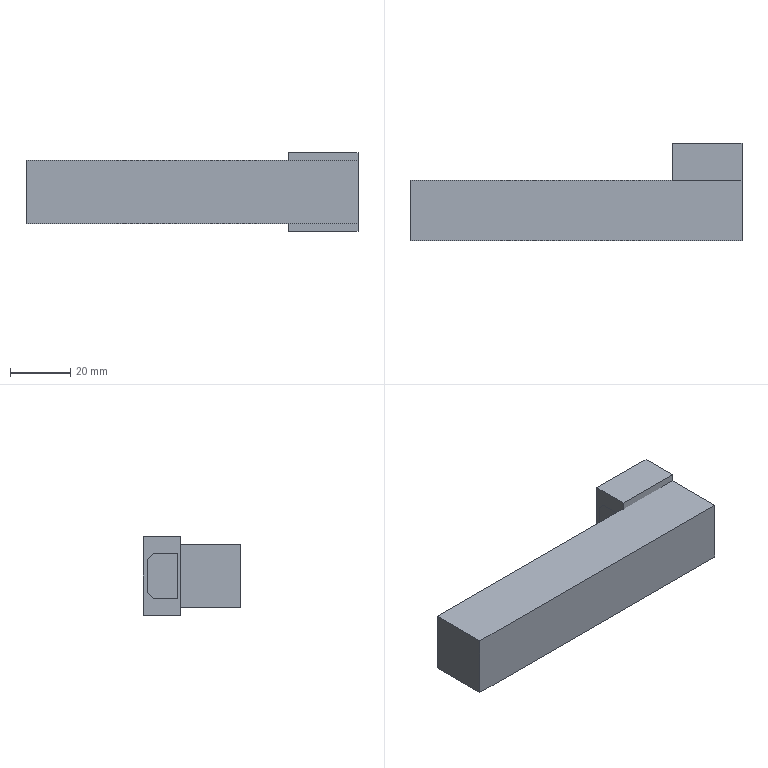NC program | NX | posted with a generic post | part box 110 x 32.2 x 26 mm
Lines 1 to 2298 of 5595, first 1795 of 2282 lines:
N10 G17 G21 G94 G90
(PLANAR_MILL , TOOL : D16C)
N12 T01 M6
N14 G54
N16 G17 G0 G90 X-64.06 Y0.06 S2300 M3
N18 G43 Z20. H1
N20 Z3.
N22 G94 G1 Z0. F800.
N24 X-48.06
N26 X50.
N28 X66.
N30 Z3.
N32 G0 Z20.
(ADAPTIVE_MILLING , TOOL : D16C)
N34 X-47.639 Y-25.487 S3500
N36 Z-9.3
N38 G1 X-47.612 Y-25.339 Z-10.237 F1500.
N40 X-47.586 Y-25.191 Z-10.608
N42 X-47.559 Y-25.044 Z-10.88
N44 X-47.533 Y-24.896 Z-11.1
N46 X-47.506 Y-24.748 Z-11.284
N48 X-47.48 Y-24.601 Z-11.442
N50 X-47.453 Y-24.453 Z-11.58
N52 X-47.427 Y-24.306 Z-11.7
N54 X-47.4 Y-24.158 Z-11.805
N56 X-47.374 Y-24.01 Z-11.898
N58 X-47.348 Y-23.863 Z-11.979
N60 X-47.321 Y-23.715 Z-12.05
N62 X-47.295 Y-23.567 Z-12.11
N64 X-47.268 Y-23.42 Z-12.162
N66 X-47.242 Y-23.272 Z-12.205
N68 X-47.215 Y-23.124 Z-12.239
N70 X-47.189 Y-22.977 Z-12.266
N72 X-47.162 Y-22.829 Z-12.285
N74 X-47.136 Y-22.681 Z-12.296
N76 X-47.109 Y-22.534 Z-12.3
N78 X-46.726 Y-20.396
N80 G3 X-48.19 Y-18.5 R1.616
N82 X-52.507 Y-18.235 R31.569
N84 G2 X-59.562 Y-14.889 R8.829
N86 X-62.127 Y-9.164 R12.797
N88 X-62.649 Y-3.232 R34.866
N90 X-62.685 Y8.843 R655.168
N92 X-59.143 Y15.242 R8.906
N94 X-53.354 Y17.682 R13.135
N96 X-47.117 Y18.161 R39.093
N98 X-37.067 Y18.2 R709.403
N100 G1 X52.988 Y18.199
N102 G2 X59.48 Y14.958 R8.794
N104 X62.125 Y9.144 R12.723
N106 X62.646 Y3.325 R34.318
N108 X62.685 Y-8.824 R620.01
N110 X59.165 Y-15.219 R8.912
N112 X53.418 Y-17.669 R13.064
N114 X47.519 Y-18.153 R36.787
N116 X37.019 Y-18.2 R709.315
N118 G1 X-45.793 Y-18.198
N120 G2 X-51.751 Y-17.939 R361.241
N122 X-59.844 Y-12.708 R10.728
N124 X-61.93 Y-6.607 R16.222
N126 X-62.365 Y0.274 R52.
N128 X-62.375 Y6.948 R189.513
N130 X-57.397 Y15.19 R10.59
N132 X-51.118 Y17.421 R15.907
N134 X-44.312 Y17.862 R50.704
N136 X-34.038 Y17.899 R728.543
N138 G1 X50.764
N140 G2 X59.63 Y12.987 R10.568
N142 X61.889 Y6.819 R15.681
N144 X62.357 Y0.203 R47.136
N146 X62.368 Y-7.033 R152.163
N148 X57.353 Y-15.217 R10.608
N150 X51.243 Y-17.401 R15.846
N152 X44.327 Y-17.862 R49.567
N154 X34.802 Y-17.899 R695.67
N156 G1 X-44.363 Y-17.897
N158 G2 X-50.474 Y-17.659 R87.545
N160 X-59.671 Y-11.376 R11.886
N162 X-61.657 Y-4.886 R18.515
N164 X-62.073 Y2.861 R65.244
N166 X-61.929 Y6.64 R22.837
N168 X-55.949 Y15.085 R11.728
N170 X-49.444 Y17.14 R18.144
N172 X-42.111 Y17.564 R60.452
N174 G1 X-31.761 Y17.599
N176 X48.813
N178 G2 X56.36 Y15.207 R11.928
N180 X60.794 Y8.696 R13.349
N182 X61.906 Y2.283 R25.894
N184 X62.05 Y-5.513 R87.082
N186 X56.042 Y-15.03 R11.703
N188 X49.505 Y-17.131 R17.992
N190 X42.06 Y-17.565 R60.128
N192 G1 X31.785 Y-17.599
N194 X-44.515 Y-17.588
N196 G2 X-49.457 Y-17.36 R55.401
N198 X-59.419 Y-10.311 R12.761
N200 X-61.353 Y-3.606 R20.225
N202 X-61.706 Y4.366 R51.532
N204 X-55.08 Y14.719 R12.499
N206 X-48.31 Y16.814 R19.379
N208 X-40.94 Y17.256 R62.006
N210 X-29.84 Y17.298 R749.749
N212 G1 X47.387 Y17.297
N214 G2 X53.58 Y16.029 R14.025
N216 X59.745 Y9.539 R13.034
N218 X61.431 Y2.877 R21.689
N220 X61.701 Y-4.424 R50.131
N222 X54.99 Y-14.767 R12.509
N224 X48.317 Y-16.812 R19.469
N226 X40.91 Y-17.256 R62.113
N228 X29.81 Y-17.298 R750.3
N230 G1 X-43.94 Y-17.299
N232 G2 X-48.686 Y-17.038 R42.716
N234 X-59.106 Y-9.454 R13.461
N236 X-61.044 Y-2.515 R21.574
N238 X-61.313 Y3.658 R33.117
N240 X-54.289 Y14.363 R13.08
N242 X-47.321 Y16.489 R20.415
N244 X-39.165 Y16.959 R67.725
N246 X-29.04 Y16.998 R721.188
N248 G1 X46.158 Y16.995
N250 G2 X51.97 Y16.024 R16.081
N252 X59.155 Y9.24 R13.423
N254 X61.051 Y2.363 R21.636
N256 X61.313 Y-3.623 R32.621
N258 X54.248 Y-14.384 R13.087
N260 X51.218 Y-15.664 R12.421
N262 X44.162 Y-16.796 R30.617
N264 X33.215 Y-16.995 R202.408
N266 G1 X28.115 Y-16.998
N268 X-43.948
N270 G2 X-49.108 Y-16.502 R26.27
N272 X-58.683 Y-8.888 R13.993
N274 X-60.688 Y-1.889 R22.084
N276 X-60.752 Y4.127 R20.912
N278 X-53.818 Y13.867 R13.457
N280 X-46.89 Y16.097 R20.532
N282 X-38.852 Y16.642 R61.265
N284 X-26.552 Y16.698 R765.35
N286 G1 X45.67 Y16.69
N288 G2 X52.27 Y15.251 R16.557
N290 G1 X52.52 Y15.191
N292 G2 X54.791 Y14.033 R9.495
N294 X57.268 Y11.365 R11.153
N296 X60.403 Y3.621 R19.669
N298 X60.886 Y-2.98 R25.727
N300 X57.099 Y-11.412 R13.467
N302 X54.022 Y-14.504 R7.94
N304 G1 X53.699 Y-14.702
N306 G2 X51.274 Y-15.49 R9.495
N308 X40.212 Y-16.618 R60.834
N310 X26.563 Y-16.698 R718.931
N312 G1 X-43.925
N314 G2 X-49.727 Y-15.818 R21.169
N316 X-58.348 Y-8.202 R14.524
N318 X-60.419 Y2.472 R21.678
N320 X-54.064 Y12.97 R13.725
N322 G1 X-52.849 Y14.034
N324 G2 X-50.577 Y15.191 R9.495
N326 X-48.103 Y15.65 R13.193
N328 X-37.295 Y16.35 R87.284
N330 X-25.146 Y16.397 R783.974
N332 G1 X44.995 Y16.396
N334 G2 X49.944 Y15.596 R22.073
N336 G1 X51.276 Y15.489
N338 X52.297 Y15.244
N340 G3 X53.497 Y15.43 R1.602
N342 G1 X54.112 Y15.801
N344 X56.844 Y17.447 Z-12.2
N346 G2 X57.413 Y17.739 R2.603 F15000.
N348 X59.229 Y17.101 R1.6
N350 G1 X62.55 Y12.119
N352 G2 X64.187 Y8.556 R12.517
N354 X65.082 Y4.692 R44.004
N356 G1 X65.33 Y3.355
N358 X65.564 Y2.016
N360 G2 X65.447 Y-5.571 R23.318
N362 X61.974 Y-13.417 R17.115
N364 G1 X57.488 Y-19.078
N366 G2 X54.972 Y-19.068 R1.6
N368 G1 X54.646 Y-18.649
N370 X52.686 Y-16.133 Z-12.3 F1500.
N372 G3 X51.274 Y-15.49 R1.603
N374 X45.161 Y-16.045 R728.767
N376 G2 X33.243 Y-16.386 R166.247
N378 G1 X25.293 Y-16.397
N380 X-43.919 Y-16.398
N382 G2 X-49.12 Y-15.508 R24.023
N384 X-50.58 Y-15.191 R10.043
N386 X-52.974 Y-13.946 R9.488
N388 X-55.554 Y-11.472 R18.869
N390 X-57.628 Y-8.549 R10.409
N392 X-59.955 Y1.385 R20.353
N394 X-57.372 Y8.945 R13.999
N396 X-56.593 Y10.291 R9.876
N398 G1 X-55.763 Y11.263
N400 X-53.986 Y13.04
N402 G3 X-54.851 Y15.749 R1.6
N404 X-55.855 Y15.599 Z-12.268 R1.733
N406 G1 X-57.859 Y14.797 Z-12.2
N408 X-60.326 Y13.81 F15000.
N410 G3 X-61.162 Y13.04 R1.603
N412 G1 X-61.98 Y11.408
N414 X-62.786 Y9.77
N416 G3 X-64.757 Y2.588 R23.064
N418 X-64.582 Y-2.243 R18.278
N420 G1 X-63.526 Y-8.432
N422 G3 X-62.902 Y-9.448 R1.602
N424 G1 X-60.84 Y-10.979
N426 X-58.912 Y-12.41 Z-12.275 F1500.
N428 G3 X-58.191 Y-12.708 Z-12.3 R1.615
N430 X-56.594 Y-10.289 R1.6
N432 G2 X-57.751 Y-8.017 R9.495
N434 X-59.297 Y-2.109 R31.269
N436 X-58.111 Y6.47 R15.528
N438 G1 X-58.059 Y6.689
N440 G3 X-59.751 Y8.499 R1.6
N442 X-60.887 Y7.911 Z-12.259 R1.617
N444 G1 X-62.067 Y6.456 Z-12.2
N446 X-63.918 Y4.174 F15000.
N448 G3 X-64.274 Y3.101 R1.603
N450 G1 X-63.966 Y-4.429
N452 G3 X-63.641 Y-5.332 R1.606
N454 G1 X-61.967 Y-7.535
N456 X-60.523 Y-9.427 Z-12.275 F1500.
N458 G3 X-59.87 Y-9.888 Z-12.3 R1.605
N460 X-57.751 Y-8.017 R1.6
N462 G2 X-58.869 Y-2.323 R50.127
N464 X-58.379 Y4.108 R17.226
N466 G3 X-58.15 Y5.501 R4.5
N468 G2 X-57.751 Y8.02 R9.498
N470 G1 X-57.334 Y9.024
N472 G3 X-59.89 Y10.82 R1.6
N474 G1 X-60.105 Y10.579 Z-12.29
N476 X-60.294 Y10.319 Z-12.28
N478 X-61.788 Y8.259 Z-12.2
N480 X-63.25 Y6.243 F15000.
N482 G3 X-63.549 Y5.436 R1.61
N484 G1 X-64.264 Y-3.186
N486 G3 X-63.892 Y-4.35 R1.602
N488 G1 X-62.082 Y-6.493
N490 X-61.446 Y-7.249 Z-12.231 F1500.
N492 X-60.803 Y-7.999 Z-12.262
N494 G3 X-59.73 Y-8.497 Z-12.3 R1.6
N496 X-58.05 Y-6.774 R1.6
N498 X-58.467 Y-2.9 R167.508
N500 G2 X-58.153 Y3.155 R23.608
N502 G1 X-58.15 Y5.199
N504 G3 X-59.745 Y6.799 R1.6
N506 X-60.973 Y6.231 Z-12.256 R1.612
N508 G1 X-62.129 Y4.861 Z-12.2
N510 X-63.987 Y2.659 F15000.
N512 G3 X-64.365 Y1.611 R1.603
N514 G1 X-64.323 Y-2.438
N516 G3 X-63.967 Y-3.428 R1.604
N518 G1 X-62.14 Y-5.686
N520 X-60.885 Y-7.227 Z-12.262 F1500.
N522 G3 X-59.833 Y-7.746 Z-12.3 R1.6
N524 X-58.109 Y-6.026 R1.6
N526 G2 X-58.172 Y-3.893 R34.44
N528 X-58.15 Y0.129 R34.348
N530 G1 Y3.241
N532 G3 X-59.75 Y4.841 R1.6
N534 X-60.975 Y4.271 Z-12.256 R1.612
N536 G1 X-62.129 Y2.897 Z-12.2
N538 X-63.99 Y0.683 F15000.
N540 G3 X-64.365 Y-0.347 R1.603
N542 G1 X-64.367 Y-0.847
N544 X-64.354 Y-1.347
N546 G3 X-63.99 Y-2.191 R1.607
N548 G1 X-62.148 Y-4.383
N550 X-61.533 Y-5.12 Z-12.23 F1500.
N552 X-60.908 Y-5.849 Z-12.26
N554 G3 X-59.779 Y-6.349 Z-12.3 R1.599
N556 X-58.15 Y-4.749 R1.6
N558 G1 Y5.501
N560 G2 X-57.751 Y8.02 R9.498
N562 X-56.593 Y10.291 R9.495
N564 G1 X-55.763 Y11.263
N566 X-53.822 Y13.203
N568 G2 X-51.759 Y14.702 R9.498
N570 X-49.334 Y15.49 R9.495
N572 X-46.196 Y15.655 R64.482
N574 X-31.016 Y16.089 R214.997
N576 G1 X-23.966 Y16.097
N578 X43.658 Y16.09
N580 G2 X48.257 Y15.59 R33.158
N582 G1 X50.001
N584 G3 X51.59 Y17.372 R1.6
N586 X50.933 Y18.49 Z-12.258 R1.617
N588 G1 X49.426 Y19.57 Z-12.2
N590 X47.811 Y20.728 F15000.
N592 G3 X46.861 Y21.028 R1.605
N594 G1 X-43.282 Y20.03
N596 X-43.489 Y20.012
N598 X-43.693 Y19.972
N600 X-45.099 Y19.58
N602 X-48.172 Y18.725 Z-12.3 F1500.
N604 G3 X-47.722 Y15.59 R1.6
N606 X-37.447 Y15.727 R305.695
N608 G2 X-22.972 Y15.797 R829.663
N610 G1 X44.428 Y15.796
N612 X46.077 Y15.59
N614 X48.289
N616 G3 X48.775 Y18.714 R1.6
N618 G1 X45.704 Y19.573 Z-12.2
N620 X44.922 Y19.794 F15000.
N622 X44.138 Y20.004
N624 X43.849 Y20.03
N626 X-39.232
N628 X-39.449 Y20.013
N630 X-39.662 Y19.971
N632 X-41.059 Y19.581
N634 X-44.131 Y18.723 Z-12.3 F1500.
N636 G3 X-43.672 Y15.59 R1.6
N638 G1 X50.001
N640 G2 X52.52 Y15.191 R9.498
N642 X54.791 Y14.033 R9.495
N644 X56.594 Y12.229 R9.495
N646 X58.612 Y8.215 R22.088
N648 X60.474 Y-1.783 R25.602
N650 X58.204 Y-9.005 R14.567
N652 G3 X57.8 Y-9.765 R4.628
N654 X58.945 Y-11.766 R1.6
N656 X60.275 Y-11.509 Z-12.256 R1.612
N658 G1 X61.724 Y-10.458 Z-12.2
N660 X64.153 Y-8.697 F15000.
N662 G3 X64.731 Y-7.908 R1.605
N664 G1 X65.118 Y-6.757
N666 X65.489 Y-5.6
N668 G3 X65.727 Y-2.15 R8.614
N670 G1 X64.194 Y9.282
N672 G3 X63.52 Y10.384 R1.602
N674 G1 X61.247 Y11.96
N676 X59.576 Y13.112 Z-12.264 F1500.
N678 G3 X58.463 Y13.327 Z-12.3 R1.6
N680 X57.262 Y11.139 R1.6
N682 G2 X58.592 Y7.424 R35.54
N684 X60.011 Y-0.144 R27.732
N686 X58.547 Y-7.21 R16.254
N688 G3 X58.067 Y-8.5 R6.221
N690 X59.065 Y-10.155 R1.6
N692 X60.42 Y-10.076 Z-12.256 R1.612
N694 G1 X61.992 Y-9.224 Z-12.2
N696 X64.161 Y-8.049 F15000.
N698 G3 X64.999 Y-6.642 R1.601
N700 G1 Y-1.24
N702 G3 X64.482 Y3.85 R25.383
N704 G1 X63.966 Y6.369
N706 G3 X63.696 Y6.984 R1.625
N708 G1 X61.994 Y9.342
N710 X60.554 Y11.331 Z-12.277 F1500.
N712 G3 X59.983 Y11.781 Z-12.3 R1.61
N714 X57.751 Y9.957 R1.6
N716 G2 X59.123 Y4.086 R181.863
N718 X58.537 Y-5.901 R18.835
N720 G3 X58.15 Y-7.362 R7.624
N722 G2 X57.751 Y-9.96 R9.467
N724 G1 X57.261 Y-11.141
N726 X57.046 Y-11.493
N728 G3 X59.742 Y-13.215 R1.6
N730 G1 X60.044 Y-12.76
N732 X61.811 Y-10.105 Z-12.2
N734 X63.213 Y-7.992 F15000.
N736 X63.774 Y-6.885
N738 X64.316 Y-5.769
N740 G3 X64.88 Y-2.352 R7.126
N742 G1 X64.264 Y5.126
N744 G3 X63.927 Y5.984 R1.607
N746 G1 X62.089 Y8.32
N748 X60.842 Y9.897 Z-12.263 F1500.
N750 G3 X59.822 Y10.429 Z-12.3 R1.6
N752 X58.05 Y8.714 R1.6
N754 X58.574 Y5.391 R30.239
N756 G2 X59.008 Y-1.285 R23.543
N758 X58.184 Y-5.786 R36.786
N760 G3 X58.15 Y-7.396 R11.777
N762 X59.746 Y-8.996 R1.6
N764 X60.973 Y-8.427 Z-12.256 R1.612
N766 G1 X62.129 Y-7.056 Z-12.2
N768 X63.988 Y-4.852 F15000.
N770 G3 X64.365 Y-3.808 R1.603
N772 G1 X64.297 Y4.714
N774 G3 X63.94 Y5.709 R1.604
N776 G1 X62.118 Y7.957
N778 X60.858 Y9.503 Z-12.263 F1500.
N780 G3 X59.813 Y10.022 Z-12.3 R1.6
N782 X58.082 Y8.303 R1.6
N784 X58.56 Y3.516 R91.879
N786 G2 X58.162 Y-4.077 R27.07
N788 G1 X58.15 Y-6.062
N790 G3 X59.75 Y-7.662 R1.6
N792 X60.975 Y-7.092 Z-12.256 R1.612
N794 G1 X62.129 Y-5.718 Z-12.2
N796 X63.99 Y-3.503 F15000.
N798 G3 X64.365 Y-2.474 R1.603
N800 G1 Y3.851
N802 G3 X63.99 Y4.881 R1.603
N804 G1 X62.148 Y7.073
N806 X61.533 Y7.81 Z-12.23 F1500.
N808 X60.908 Y8.539 Z-12.26
N810 G3 X59.779 Y9.039 Z-12.3 R1.599
N812 X58.15 Y7.439 R1.6
N814 X58.294 Y3.052 R67.239
N816 G2 X58.15 Y-1.367 R32.924
N818 G1 Y-4.226
N820 G3 X60.913 Y-5.324 R1.6
N822 X61.306 Y-4.631 Z-12.275 R1.812
N824 G1 X62.133 Y-2.393 Z-12.2
N826 X63.125 Y0.294 F15000.
N828 G3 X63.224 Y1.053 R1.961
N830 X63.125 Y1.607 R1.667
N832 G1 X62.141 Y4.271
N834 X61.251 Y6.681 Z-12.281 F1500.
N836 G3 X60.93 Y7.207 Z-12.3 R1.636
N838 X58.15 Y6.127 R1.6
N840 G1 Y-7.441
N842 G2 X57.751 Y-9.96 R9.498
N844 X56.593 Y-12.231 R9.495
N846 X54.789 Y-14.034 R9.495
N848 X52.517 Y-15.191 R9.495
N850 X49.999 Y-15.59 R9.5
N852 G3 X44.112 Y-15.817 R77.937
N854 G2 X29.491 Y-16.093 R278.819
N856 G1 X24.166 Y-16.097
N858 X-41.883
N860 G2 X-47.063 Y-15.59 R31.033
N862 X-49.182 Y-15.502 R15.499
N864 G3 X-50.871 Y-17.438 R1.6
N866 X-50.091 Y-18.5 Z-12.258 R1.685
N868 G1 X-48.582 Y-19.542 Z-12.2
N870 X-46.968 Y-20.656 F15000.
N872 G3 X-46.043 Y-20.939 R1.605
N874 G1 X44.134 Y-20.03
N876 X44.342 Y-20.012
N878 X44.547 Y-19.972
N880 X45.952 Y-19.581
N882 X49.024 Y-18.726 Z-12.3 F1500.
N884 G3 X48.574 Y-15.59 R1.6
N886 X37.854 Y-15.727 R322.207
N888 G2 X23.155 Y-15.797 R840.773
N890 G1 X-41.92 Y-15.796
N892 G2 X-44.488 Y-15.59 R78.283
N894 G1 X-47.076
N896 G3 X-47.562 Y-18.714 R1.6
N898 G1 X-44.49 Y-19.573 Z-12.2
N900 X-43.709 Y-19.794 F15000.
N902 X-42.925 Y-20.004
N904 X-42.636 Y-20.03
N906 X39.784
N908 X40.001 Y-20.013
N910 X40.215 Y-19.971
N912 X41.611 Y-19.581
N914 X44.683 Y-18.723 Z-12.3 F1500.
N916 G3 X44.224 Y-15.59 R1.6
N918 G1 X-48.061
N920 G2 X-50.58 Y-15.191 R9.498
N922 X-52.851 Y-14.033 R9.495
N924 G1 X-53.823 Y-13.203
N926 X-55.573 Y-11.452
N928 G3 X-57.723 Y-11.331 R1.616
N930 G1 X-59.641 Y-12.859
N932 X-59.758 Y-12.953 Z-12.296
N934 X-59.875 Y-13.046 Z-12.285
N936 X-59.993 Y-13.14 Z-12.266
N938 X-60.11 Y-13.233 Z-12.239
N940 X-60.227 Y-13.327 Z-12.205
N942 X-60.345 Y-13.42 Z-12.162
N944 X-60.462 Y-13.514 Z-12.11
N946 X-60.579 Y-13.607 Z-12.05
N948 X-60.697 Y-13.701 Z-11.979
N950 X-60.814 Y-13.794 Z-11.898
N952 X-60.931 Y-13.888 Z-11.805
N954 X-61.049 Y-13.981 Z-11.7
N956 X-61.166 Y-14.075 Z-11.58
N958 X-61.283 Y-14.168 Z-11.442
N960 X-61.4 Y-14.262 Z-11.284
N962 X-61.518 Y-14.355 Z-11.1
N964 X-61.635 Y-14.449 Z-10.88
N966 X-61.752 Y-14.542 Z-10.608
N968 X-61.87 Y-14.636 Z-10.237
N970 X-61.987 Y-14.729 Z-9.3
N972 G0 Z20.
N974 M5
(PLANAR_MILL_1 , TOOL : D14J)
N976 T02 M6
N978 G54
N980 G17 G0 G90 X60.239 Y-14.527 S3000 M3
N982 G43 Z20. H2
N984 Z-10.3
N986 G94 G1 Z-12.3 F600.
N988 G41 X59.747 Y-14.44 D2
N990 X49.998
N992 X-48.06
N994 G2 X-53.01 Y-12.39 R7.
N996 G1 X-54.95 Y-10.45
N998 G2 X-57. Y-5.5 R7.
N1000 G1 Y5.5
N1002 G2 X-54.95 Y10.45 R7.
N1004 G1 X-53.01 Y12.39
N1006 G2 X-48.06 Y14.44 R7.
N1008 G1 X50.
N1010 G2 X57. Y7.44 R7.
N1012 G1 Y-7.438
N1014 Y-17.187
N1016 G40
N1018 X57.087 Y-17.679
N1020 Z-10.3
N1022 G0 Z20.
N1024 X60.239 Y-14.527
N1026 Z-10.3
N1028 G1 Z-12.3
N1030 G41 X59.747 Y-14.44
N1032 X49.998
N1034 X-48.06
N1036 G2 X-53.01 Y-12.39 R7.
N1038 G1 X-54.95 Y-10.45
N1040 G2 X-57. Y-5.5 R7.
N1042 G1 Y5.5
N1044 G2 X-54.95 Y10.45 R7.
N1046 G1 X-53.01 Y12.39
N1048 G2 X-48.06 Y14.44 R7.
N1050 G1 X50.
N1052 G2 X57. Y7.44 R7.
N1054 G1 Y-7.438
N1056 Y-17.187
N1058 G40
N1060 X57.087 Y-17.679
N1062 Z-10.3
N1064 G0 Z20.
N1066 M5
(PLANAR_MILL_2 , TOOL : D4C)
N1068 T03 M6
N1070 G54
N1072 G17 G0 G90 X-43.261 Y-1.15 S3500 M3
N1074 G43 Z20. H3
N1076 Z0.5
N1078 G94 G1 X22.264 Z0.386 F2000.
N1080 X22.834 Y-0.834 Z0.385
N1082 X23.15 Y-0.264 Z0.383
N1084 Y0.
N1086 Y0.264 Z0.382
N1088 X22.834 Y0.834 Z0.381
N1090 X22.264 Y1.15 Z0.38
N1092 X-43.264 Z0.266
N1094 X-43.834 Y0.834 Z0.265
N1096 X-44.15 Y0.264 Z0.264
N1098 Y-0.264 Z0.263
N1100 X-43.834 Y-0.834 Z0.261
N1102 X-43.264 Y-1.15 Z0.26
N1104 X22.264 Z0.146
N1106 X22.834 Y-0.834 Z0.145
N1108 X23.15 Y-0.264 Z0.144
N1110 Y0. Z0.143
N1112 Y0.264
N1114 X22.834 Y0.834 Z0.142
N1116 X22.264 Y1.15 Z0.14
N1118 X-43.264 Z0.026
N1120 X-43.834 Y0.834 Z0.025
N1122 X-44.15 Y0.264 Z0.024
N1124 Y-0.264 Z0.023
N1126 X-43.834 Y-0.834 Z0.022
N1128 X-43.264 Y-1.15 Z0.021
N1130 X22.264 Z-0.094
N1132 X22.834 Y-0.834 Z-0.095
N1134 X23.15 Y-0.264 Z-0.096
N1136 Y0.
N1138 Y0.264 Z-0.097
N1140 X22.834 Y0.834 Z-0.098
N1142 X22.264 Y1.15 Z-0.099
N1144 X-43.264 Z-0.214
N1146 X-43.834 Y0.834 Z-0.215
N1148 X-44.15 Y0.264 Z-0.216
N1150 Y-0.264 Z-0.217
N1152 X-43.834 Y-0.834 Z-0.218
N1154 X-43.264 Y-1.15 Z-0.219
N1156 X22.264 Z-0.333
N1158 X22.834 Y-0.834 Z-0.335
N1160 X23.15 Y-0.264 Z-0.336
N1162 Y0.
N1164 Y0.264 Z-0.337
N1166 X22.834 Y0.834 Z-0.338
N1168 X22.264 Y1.15 Z-0.339
N1170 X-43.264 Z-0.453
N1172 X-43.834 Y0.834 Z-0.454
N1174 X-44.15 Y0.264 Z-0.456
N1176 Y-0.264
N1178 X-43.834 Y-0.834 Z-0.458
N1180 X-43.264 Y-1.15 Z-0.459
N1182 X22.264 Z-0.573
N1184 X22.834 Y-0.834 Z-0.574
N1186 X23.15 Y-0.264 Z-0.575
N1188 Y0. Z-0.576
N1190 Y0.264
N1192 X22.834 Y0.834 Z-0.577
N1194 X22.264 Y1.15 Z-0.579
N1196 X-43.264 Z-0.693
N1198 X-43.834 Y0.834 Z-0.694
N1200 X-44.15 Y0.264 Z-0.695
N1202 Y-0.264 Z-0.696
N1204 X-43.834 Y-0.834 Z-0.697
N1206 X-43.264 Y-1.15 Z-0.698
N1208 X22.264 Z-0.813
N1210 X22.834 Y-0.834 Z-0.814
N1212 X23.15 Y-0.264 Z-0.815
N1214 Y0. Z-0.816
N1216 Y0.264
N1218 X22.834 Y0.834 Z-0.817
N1220 X22.264 Y1.15 Z-0.818
N1222 X-43.264 Z-0.933
N1224 X-43.834 Y0.834 Z-0.934
N1226 X-44.15 Y0.264 Z-0.935
N1228 Y-0.264 Z-0.936
N1230 X-43.834 Y-0.834 Z-0.937
N1232 X-43.264 Y-1.15 Z-0.938
N1234 X22.264 Z-1.052
N1236 X22.834 Y-0.834 Z-1.054
N1238 X23.15 Y-0.264 Z-1.055
N1240 Y0.
N1242 Y0.264 Z-1.056
N1244 X22.834 Y0.834 Z-1.057
N1246 X22.264 Y1.15 Z-1.058
N1248 X-43.264 Z-1.172
N1250 X-43.834 Y0.834 Z-1.173
N1252 X-44.15 Y0.264 Z-1.175
N1254 Y-0.264
N1256 X-43.834 Y-0.834 Z-1.177
N1258 X-43.264 Y-1.15 Z-1.178
N1260 X22.264 Z-1.292
N1262 X22.834 Y-0.834 Z-1.293
N1264 X23.15 Y-0.264 Z-1.294
N1266 Y0. Z-1.295
N1268 Y0.264
N1270 X22.834 Y0.834 Z-1.296
N1272 X22.264 Y1.15 Z-1.298
N1274 X-43.264 Z-1.412
N1276 X-43.834 Y0.834 Z-1.413
N1278 X-44.15 Y0.264 Z-1.414
N1280 Y-0.264 Z-1.415
N1282 X-43.834 Y-0.834 Z-1.416
N1284 X-43.264 Y-1.15 Z-1.417
N1286 X22.264 Z-1.532
N1288 X22.834 Y-0.834 Z-1.533
N1290 X23.15 Y-0.264 Z-1.534
N1292 Y0. Z-1.535
N1294 Y0.264
N1296 X22.834 Y0.834 Z-1.536
N1298 X22.264 Y1.15 Z-1.537
N1300 X-43.264 Z-1.652
N1302 X-43.834 Y0.834 Z-1.653
N1304 X-44.15 Y0.264 Z-1.654
N1306 Y-0.264 Z-1.655
N1308 X-43.834 Y-0.834 Z-1.656
N1310 X-43.264 Y-1.15 Z-1.657
N1312 X22.264 Z-1.772
N1314 X22.834 Y-0.834 Z-1.773
N1316 X23.15 Y-0.264 Z-1.774
N1318 Y0.
N1320 Y0.264 Z-1.775
N1322 X22.834 Y0.834 Z-1.776
N1324 X22.264 Y1.15 Z-1.777
N1326 X-43.264 Z-1.891
N1328 X-43.834 Y0.834 Z-1.892
N1330 X-44.15 Y0.264 Z-1.894
N1332 Y-0.264 Z-1.895
N1334 X-43.834 Y-0.834 Z-1.896
N1336 X-43.264 Y-1.15 Z-1.897
N1338 X22.264 Z-2.011
N1340 X22.834 Y-0.834 Z-2.012
N1342 X23.15 Y-0.264 Z-2.013
N1344 Y0. Z-2.014
N1346 Y0.264
N1348 X22.834 Y0.834 Z-2.016
N1350 X22.264 Y1.15 Z-2.017
N1352 X-43.264 Z-2.131
N1354 X-43.834 Y0.834 Z-2.132
N1356 X-44.15 Y0.264 Z-2.133
N1358 Y-0.264 Z-2.134
N1360 X-43.834 Y-0.834 Z-2.135
N1362 X-43.264 Y-1.15 Z-2.136
N1364 X22.264 Z-2.251
N1366 X22.834 Y-0.834 Z-2.252
N1368 X23.15 Y-0.264 Z-2.253
N1370 Y0. Z-2.254
N1372 Y0.264
N1374 X22.834 Y0.834 Z-2.255
N1376 X22.264 Y1.15 Z-2.256
N1378 X-43.264 Z-2.371
N1380 X-43.834 Y0.834 Z-2.372
N1382 X-44.15 Y0.264 Z-2.373
N1384 Y-0.264 Z-2.374
N1386 X-43.834 Y-0.834 Z-2.375
N1388 X-43.264 Y-1.15 Z-2.376
N1390 X22.264 Z-2.491
N1392 X22.834 Y-0.834 Z-2.492
N1394 X23.15 Y-0.264 Z-2.493
N1396 Y0.
N1398 Y0.264 Z-2.494
N1400 X22.834 Y0.834 Z-2.495
N1402 X22.264 Y1.15 Z-2.496
N1404 X-43.264 Z-2.61
N1406 X-43.834 Y0.834 Z-2.612
N1408 X-44.15 Y0.264 Z-2.613
N1410 Y-0.264 Z-2.614
N1412 X-43.834 Y-0.834 Z-2.615
N1414 X-43.264 Y-1.15 Z-2.616
N1416 X22.264 Z-2.73
N1418 X22.834 Y-0.834 Z-2.731
N1420 X23.15 Y-0.264 Z-2.733
N1422 Y0.
N1424 Y0.264
N1426 X22.834 Y0.834 Z-2.735
N1428 X22.264 Y1.15 Z-2.736
N1430 X-43.264 Z-2.85
N1432 X-43.834 Y0.834 Z-2.851
N1434 X-44.15 Y0.264 Z-2.852
N1436 Y-0.264 Z-2.853
N1438 X-43.834 Y-0.834 Z-2.854
N1440 X-43.264 Y-1.15 Z-2.856
N1442 X22.264 Z-2.97
N1444 X22.834 Y-0.834 Z-2.971
N1446 X23.15 Y-0.264 Z-2.972
N1448 Y0. Z-2.973
N1450 Y0.264
N1452 X22.834 Y0.834 Z-2.974
N1454 X22.264 Y1.15 Z-2.975
N1456 X-43.264 Z-3.09
N1458 X-43.834 Y0.834 Z-3.091
N1460 X-44.15 Y0.264 Z-3.092
N1462 Y-0.264 Z-3.093
N1464 X-43.834 Y-0.834 Z-3.094
N1466 X-43.264 Y-1.15 Z-3.095
N1468 X22.264 Z-3.21
N1470 X22.834 Y-0.834 Z-3.211
N1472 X23.15 Y-0.264 Z-3.212
N1474 Y0.
N1476 Y0.264 Z-3.213
N1478 X22.834 Y0.834 Z-3.214
N1480 X22.264 Y1.15 Z-3.215
N1482 X-43.264 Z-3.329
N1484 X-43.834 Y0.834 Z-3.331
N1486 X-44.15 Y0.264 Z-3.332
N1488 Y-0.264 Z-3.333
N1490 X-43.834 Y-0.834 Z-3.334
N1492 X-43.264 Y-1.15 Z-3.335
N1494 X22.264 Z-3.449
N1496 X22.834 Y-0.834 Z-3.45
N1498 X23.15 Y-0.264 Z-3.452
N1500 Y0.
N1502 Y0.264
N1504 X22.834 Y0.834 Z-3.454
N1506 X22.264 Y1.15 Z-3.455
N1508 X-43.264 Z-3.569
N1510 X-43.834 Y0.834 Z-3.57
N1512 X-44.15 Y0.264 Z-3.571
N1514 Y-0.264 Z-3.572
N1516 X-43.834 Y-0.834 Z-3.573
N1518 X-43.264 Y-1.15 Z-3.575
N1520 X22.264 Z-3.689
N1522 X22.834 Y-0.834 Z-3.69
N1524 X23.15 Y-0.264 Z-3.691
N1526 Y0. Z-3.692
N1528 Y0.264
N1530 X22.834 Y0.834 Z-3.693
N1532 X22.264 Y1.15 Z-3.694
N1534 X-43.264 Z-3.809
N1536 X-43.834 Y0.834 Z-3.81
N1538 X-44.15 Y0.264 Z-3.811
N1540 Y-0.264 Z-3.812
N1542 X-43.834 Y-0.834 Z-3.813
N1544 X-43.264 Y-1.15 Z-3.814
N1546 X22.264 Z-3.929
N1548 X22.834 Y-0.834 Z-3.93
N1550 X23.15 Y-0.264 Z-3.931
N1552 Y0.
N1554 Y0.264 Z-3.932
N1556 X22.834 Y0.834 Z-3.933
N1558 X22.264 Y1.15 Z-3.934
N1560 X-43.264 Z-4.048
N1562 X-43.834 Y0.834 Z-4.05
N1564 X-44.15 Y0.264 Z-4.051
N1566 Y-0.264 Z-4.052
N1568 X-43.834 Y-0.834 Z-4.053
N1570 X-43.264 Y-1.15 Z-4.054
N1572 X22.264 Z-4.168
N1574 X22.834 Y-0.834 Z-4.169
N1576 X23.15 Y-0.264 Z-4.171
N1578 Y0.
N1580 Y0.264 Z-4.172
N1582 X22.834 Y0.834 Z-4.173
N1584 X22.264 Y1.15 Z-4.174
N1586 X-43.264 Z-4.288
N1588 X-43.834 Y0.834 Z-4.289
N1590 X-44.15 Y0.264 Z-4.29
N1592 Y-0.264 Z-4.291
N1594 X-43.834 Y-0.834 Z-4.292
N1596 X-43.264 Y-1.15 Z-4.294
N1598 X22.264 Z-4.408
N1600 X22.834 Y-0.834 Z-4.409
N1602 X23.15 Y-0.264 Z-4.41
N1604 Y0. Z-4.411
N1606 Y0.264
N1608 X22.834 Y0.834 Z-4.412
N1610 X22.264 Y1.15 Z-4.413
N1612 X-43.264 Z-4.528
N1614 X-43.834 Y0.834 Z-4.529
N1616 X-44.15 Y0.264 Z-4.53
N1618 Y-0.264 Z-4.531
N1620 X-43.834 Y-0.834 Z-4.532
N1622 X-43.264 Y-1.15 Z-4.533
N1624 X22.264 Z-4.648
N1626 X22.834 Y-0.834 Z-4.649
N1628 X23.15 Y-0.264 Z-4.65
N1630 Y0.
N1632 Y0.264 Z-4.651
N1634 X22.834 Y0.834 Z-4.652
N1636 X22.264 Y1.15 Z-4.653
N1638 X-43.264 Z-4.768
N1640 X-43.834 Y0.834 Z-4.769
N1642 X-44.15 Y0.264 Z-4.77
N1644 Y-0.264 Z-4.771
N1646 X-43.834 Y-0.834 Z-4.772
N1648 X-43.264 Y-1.15 Z-4.773
N1650 X22.264 Z-4.887
N1652 X22.834 Y-0.834 Z-4.889
N1654 X23.15 Y-0.264 Z-4.89
N1656 Y0.
N1658 Y0.264 Z-4.891
N1660 X22.834 Y0.834 Z-4.892
N1662 X22.264 Y1.15 Z-4.893
N1664 X-43.264 Z-5.007
N1666 X-43.834 Y0.834 Z-5.008
N1668 X-44.15 Y0.264 Z-5.009
N1670 Y-0.264 Z-5.01
N1672 X-43.834 Y-0.834 Z-5.012
N1674 X-43.264 Y-1.15 Z-5.013
N1676 X22.264 Z-5.127
N1678 X22.834 Y-0.834 Z-5.128
N1680 X23.15 Y-0.264 Z-5.129
N1682 Y0. Z-5.13
N1684 Y0.264
N1686 X22.834 Y0.834 Z-5.131
N1688 X22.264 Y1.15 Z-5.133
N1690 X-43.264 Z-5.247
N1692 X-43.834 Y0.834 Z-5.248
N1694 X-44.15 Y0.264 Z-5.249
N1696 Y-0.264 Z-5.25
N1698 X-43.834 Y-0.834 Z-5.251
N1700 X-43.264 Y-1.15 Z-5.252
N1702 X22.264 Z-5.367
N1704 X22.834 Y-0.834 Z-5.368
N1706 X23.15 Y-0.264 Z-5.369
N1708 Y0.
N1710 Y0.264 Z-5.37
N1712 X22.834 Y0.834 Z-5.371
N1714 X22.264 Y1.15 Z-5.372
N1716 X-43.264 Z-5.487
N1718 X-43.834 Y0.834 Z-5.488
N1720 X-44.15 Y0.264 Z-5.489
N1722 Y-0.264 Z-5.49
N1724 X-43.834 Y-0.834 Z-5.491
N1726 X-43.264 Y-1.15 Z-5.492
N1728 X22.264 Z-5.606
N1730 X22.834 Y-0.834 Z-5.608
N1732 X23.15 Y-0.264 Z-5.609
N1734 Y0.
N1736 Y0.264 Z-5.61
N1738 X22.834 Y0.834 Z-5.611
N1740 X22.264 Y1.15 Z-5.612
N1742 X-43.264 Z-5.726
N1744 X-43.834 Y0.834 Z-5.727
N1746 X-44.15 Y0.264 Z-5.729
N1748 Y-0.264
N1750 X-43.834 Y-0.834 Z-5.731
N1752 X-43.264 Y-1.15 Z-5.732
N1754 X22.264 Z-5.846
N1756 X22.834 Y-0.834 Z-5.847
N1758 X23.15 Y-0.264 Z-5.848
N1760 Y0. Z-5.849
N1762 Y0.264
N1764 X22.834 Y0.834 Z-5.85
N1766 X22.264 Y1.15 Z-5.852
N1768 X-43.264 Z-5.966
N1770 X-43.834 Y0.834 Z-5.967
N1772 X-44.15 Y0.264 Z-5.968
N1774 Y-0.264 Z-5.969
N1776 X-43.834 Y-0.834 Z-5.97
N1778 X-43.264 Y-1.15 Z-5.971
N1780 X22.264 Z-6.086
N1782 X22.834 Y-0.834 Z-6.087
N1784 X23.15 Y-0.264 Z-6.088
N1786 Y0. Z-6.089
N1788 Y0.264
N1790 X22.834 Y0.834 Z-6.09
N1792 X22.264 Y1.15 Z-6.091
N1794 X-43.264 Z-6.206
N1796 X-43.834 Y0.834 Z-6.207
N1798 X-44.15 Y0.264 Z-6.208
N1800 Y-0.264 Z-6.209
N1802 X-43.834 Y-0.834 Z-6.21
N1804 X-43.264 Y-1.15 Z-6.211
N1806 X22.264 Z-6.325
N1808 X22.834 Y-0.834 Z-6.327
N1810 X23.15 Y-0.264 Z-6.328
N1812 Y0.
N1814 Y0.264 Z-6.329
N1816 X22.834 Y0.834 Z-6.33
N1818 X22.264 Y1.15 Z-6.331
N1820 X-43.264 Z-6.445
N1822 X-43.834 Y0.834 Z-6.446
N1824 X-44.15 Y0.264 Z-6.448
N1826 Y-0.264
N1828 X-43.834 Y-0.834 Z-6.45
N1830 X-43.264 Y-1.15 Z-6.451
N1832 X22.264 Z-6.565
N1834 X22.834 Y-0.834 Z-6.566
N1836 X23.15 Y-0.264 Z-6.567
N1838 Y0. Z-6.568
N1840 Y0.264
N1842 X22.834 Y0.834 Z-6.569
N1844 X22.264 Y1.15 Z-6.571
N1846 X-43.264 Z-6.685
N1848 X-43.834 Y0.834 Z-6.686
N1850 X-44.15 Y0.264 Z-6.687
N1852 Y-0.264 Z-6.688
N1854 X-43.834 Y-0.834 Z-6.689
N1856 X-43.264 Y-1.15 Z-6.69
N1858 X22.264 Z-6.805
N1860 X22.834 Y-0.834 Z-6.806
N1862 X23.15 Y-0.264 Z-6.807
N1864 Y0. Z-6.808
N1866 Y0.264
N1868 X22.834 Y0.834 Z-6.809
N1870 X22.264 Y1.15 Z-6.81
N1872 X-43.264 Z-6.925
N1874 X-43.834 Y0.834 Z-6.926
N1876 X-44.15 Y0.264 Z-6.927
N1878 Y-0.264 Z-6.928
N1880 X-43.834 Y-0.834 Z-6.929
N1882 X-43.264 Y-1.15 Z-6.93
N1884 X22.264 Z-7.045
N1886 X22.834 Y-0.834 Z-7.046
N1888 X23.15 Y-0.264 Z-7.047
N1890 Y0.
N1892 Y0.264 Z-7.048
N1894 X22.834 Y0.834 Z-7.049
N1896 X22.264 Y1.15 Z-7.05
N1898 X-43.264 Z-7.164
N1900 X-43.834 Y0.834 Z-7.165
N1902 X-44.15 Y0.264 Z-7.167
N1904 Y-0.264 Z-7.168
N1906 X-43.834 Y-0.834 Z-7.169
N1908 X-43.264 Y-1.15 Z-7.17
N1910 X22.264 Z-7.284
N1912 X22.834 Y-0.834 Z-7.285
N1914 X23.15 Y-0.264 Z-7.286
N1916 Y0. Z-7.287
N1918 Y0.264
N1920 X22.834 Y0.834 Z-7.289
N1922 X22.264 Y1.15 Z-7.29
N1924 X-43.264 Z-7.404
N1926 X-43.834 Y0.834 Z-7.405
N1928 X-44.15 Y0.264 Z-7.406
N1930 Y-0.264 Z-7.407
N1932 X-43.834 Y-0.834 Z-7.408
N1934 X-43.264 Y-1.15 Z-7.409
N1936 X22.264 Z-7.524
N1938 X22.834 Y-0.834 Z-7.525
N1940 X23.15 Y-0.264 Z-7.526
N1942 Y0. Z-7.527
N1944 Y0.264
N1946 X22.834 Y0.834 Z-7.528
N1948 X22.264 Y1.15 Z-7.529
N1950 X-43.264 Z-7.644
N1952 X-43.834 Y0.834 Z-7.645
N1954 X-44.15 Y0.264 Z-7.646
N1956 Y-0.264 Z-7.647
N1958 X-43.834 Y-0.834 Z-7.648
N1960 X-43.264 Y-1.15 Z-7.649
N1962 X22.264 Z-7.764
N1964 X22.834 Y-0.834 Z-7.765
N1966 X23.15 Y-0.264 Z-7.766
N1968 Y0.
N1970 Y0.264 Z-7.767
N1972 X22.834 Y0.834 Z-7.768
N1974 X22.264 Y1.15 Z-7.769
N1976 X-43.264 Z-7.883
N1978 X-43.834 Y0.834 Z-7.885
N1980 X-44.15 Y0.264 Z-7.886
N1982 Y-0.264 Z-7.887
N1984 X-43.834 Y-0.834 Z-7.888
N1986 X-43.264 Y-1.15 Z-7.889
N1988 X22.264 Z-8.003
N1990 X22.834 Y-0.834 Z-8.004
N1992 X23.15 Y-0.264 Z-8.006
N1994 Y0.
N1996 Y0.264
N1998 X22.834 Y0.834 Z-8.008
N2000 X22.264 Y1.15 Z-8.009
N2002 X-43.264 Z-8.123
N2004 X-43.834 Y0.834 Z-8.124
N2006 X-44.15 Y0.264 Z-8.125
N2008 Y-0.264 Z-8.126
N2010 X-43.834 Y-0.834 Z-8.127
N2012 X-43.264 Y-1.15 Z-8.129
N2014 X22.264 Z-8.243
N2016 X22.834 Y-0.834 Z-8.244
N2018 X23.15 Y-0.264 Z-8.245
N2020 Y0. Z-8.246
N2022 Y0.264
N2024 X22.834 Y0.834 Z-8.247
N2026 X22.264 Y1.15 Z-8.248
N2028 X-43.264 Z-8.363
N2030 X-43.834 Y0.834 Z-8.364
N2032 X-44.15 Y0.264 Z-8.365
N2034 Y-0.264 Z-8.366
N2036 X-43.834 Y-0.834 Z-8.367
N2038 X-43.264 Y-1.15 Z-8.368
N2040 X22.264 Z-8.483
N2042 X22.834 Y-0.834 Z-8.484
N2044 X23.15 Y-0.264 Z-8.485
N2046 Y0.
N2048 Y0.264 Z-8.486
N2050 X22.834 Y0.834 Z-8.487
N2052 X22.264 Y1.15 Z-8.488
N2054 X-43.264 Z-8.602
N2056 X-43.834 Y0.834 Z-8.604
N2058 X-44.15 Y0.264 Z-8.605
N2060 Y-0.264 Z-8.606
N2062 X-43.834 Y-0.834 Z-8.607
N2064 X-43.264 Y-1.15 Z-8.608
N2066 X22.264 Z-8.722
N2068 X22.834 Y-0.834 Z-8.723
N2070 X23.15 Y-0.264 Z-8.725
N2072 Y0.
N2074 Y0.264
N2076 X22.834 Y0.834 Z-8.727
N2078 X22.264 Y1.15 Z-8.728
N2080 X-43.264 Z-8.842
N2082 X-43.834 Y0.834 Z-8.843
N2084 X-44.15 Y0.264 Z-8.844
N2086 Y-0.264 Z-8.845
N2088 X-43.834 Y-0.834 Z-8.846
N2090 X-43.264 Y-1.15 Z-8.848
N2092 X22.264 Z-8.962
N2094 X22.834 Y-0.834 Z-8.963
N2096 X23.15 Y-0.264 Z-8.964
N2098 Y0. Z-8.965
N2100 Y0.264
N2102 X22.834 Y0.834 Z-8.966
N2104 X22.264 Y1.15 Z-8.967
N2106 X-43.264 Z-9.082
N2108 X-43.834 Y0.834 Z-9.083
N2110 X-44.15 Y0.264 Z-9.084
N2112 Y-0.264 Z-9.085
N2114 X-43.834 Y-0.834 Z-9.086
N2116 X-43.264 Y-1.15 Z-9.087
N2118 X22.264 Z-9.202
N2120 X22.834 Y-0.834 Z-9.203
N2122 X23.15 Y-0.264 Z-9.204
N2124 Y0.
N2126 Y0.264 Z-9.205
N2128 X22.834 Y0.834 Z-9.206
N2130 X22.264 Y1.15 Z-9.207
N2132 X-43.264 Z-9.321
N2134 X-43.834 Y0.834 Z-9.323
N2136 X-44.15 Y0.264 Z-9.324
N2138 Y-0.264 Z-9.325
N2140 X-43.834 Y-0.834 Z-9.326
N2142 X-43.264 Y-1.15 Z-9.327
N2144 X22.264 Z-9.441
N2146 X22.834 Y-0.834 Z-9.442
N2148 X23.15 Y-0.264 Z-9.444
N2150 Y0.
N2152 Y0.264 Z-9.445
N2154 X22.834 Y0.834 Z-9.446
N2156 X22.264 Y1.15 Z-9.447
N2158 X-43.264 Z-9.561
N2160 X-43.834 Y0.834 Z-9.562
N2162 X-44.15 Y0.264 Z-9.563
N2164 Y-0.264 Z-9.564
N2166 X-43.834 Y-0.834 Z-9.565
N2168 X-43.264 Y-1.15 Z-9.567
N2170 X22.264 Z-9.681
N2172 X22.834 Y-0.834 Z-9.682
N2174 X23.15 Y-0.264 Z-9.683
N2176 Y0. Z-9.684
N2178 Y0.264
N2180 X22.834 Y0.834 Z-9.685
N2182 X22.264 Y1.15 Z-9.686
N2184 X-43.264 Z-9.801
N2186 X-43.834 Y0.834 Z-9.802
N2188 X-44.15 Y0.264 Z-9.803
N2190 Y-0.264 Z-9.804
N2192 X-43.834 Y-0.834 Z-9.805
N2194 X-43.264 Y-1.15 Z-9.806
N2196 X22.264 Z-9.921
N2198 X22.834 Y-0.834 Z-9.922
N2200 X23.15 Y-0.264 Z-9.923
N2202 Y0.
N2204 Y0.264 Z-9.924
N2206 X22.834 Y0.834 Z-9.925
N2208 X22.264 Y1.15 Z-9.926
N2210 X-43.264 Z-10.041
N2212 X-43.834 Y0.834 Z-10.042
N2214 X-44.15 Y0.264 Z-10.043
N2216 Y-0.264 Z-10.044
N2218 X-43.834 Y-0.834 Z-10.045
N2220 X-43.264 Y-1.15 Z-10.046
N2222 X22.264 Z-10.16
N2224 X22.834 Y-0.834 Z-10.162
N2226 X23.15 Y-0.264 Z-10.163
N2228 Y0.
N2230 Y0.264 Z-10.164
N2232 X22.834 Y0.834 Z-10.165
N2234 X22.264 Y1.15 Z-10.166
N2236 X-43.264 Z-10.28
N2238 X-43.834 Y0.834 Z-10.281
N2240 X-44.15 Y0.264 Z-10.282
N2242 Y-0.264 Z-10.283
N2244 X-43.834 Y-0.834 Z-10.285
N2246 X-43.264 Y-1.15 Z-10.286
N2248 X22.264 Z-10.4
N2250 X22.834 Y-0.834 Z-10.401
N2252 X23.15 Y-0.264 Z-10.402
N2254 Y0. Z-10.403
N2256 Y0.264
N2258 X22.834 Y0.834 Z-10.404
N2260 X22.264 Y1.15 Z-10.406
N2262 X-43.264 Z-10.52
N2264 X-43.834 Y0.834 Z-10.521
N2266 X-44.15 Y0.264 Z-10.522
N2268 Y-0.264 Z-10.523
N2270 X-43.834 Y-0.834 Z-10.524
N2272 X-43.264 Y-1.15 Z-10.525
N2274 X22.264 Z-10.64
N2276 X22.834 Y-0.834 Z-10.641
N2278 X23.15 Y-0.264 Z-10.642
N2280 Y0.
N2282 Y0.264 Z-10.643
N2284 X22.834 Y0.834 Z-10.644
N2286 X22.264 Y1.15 Z-10.645
N2288 X-43.264 Z-10.76
N2290 X-43.834 Y0.834 Z-10.761
N2292 X-44.15 Y0.264 Z-10.762
N2294 Y-0.264 Z-10.763
N2296 X-43.834 Y-0.834 Z-10.764
N2298 X-43.264 Y-1.15 Z-10.765
N2300 X22.264 Z-10.879
N2302 X22.834 Y-0.834 Z-10.881
N2304 X23.15 Y-0.264 Z-10.882
N2306 Y0.
N2308 Y0.264 Z-10.883
N2310 X22.834 Y0.834 Z-10.884
N2312 X22.264 Y1.15 Z-10.885
N2314 X-43.264 Z-10.999
N2316 X-43.834 Y0.834 Z-11.
N2318 X-44.15 Y0.264 Z-11.002
N2320 Y-0.264
N2322 X-43.834 Y-0.834 Z-11.004
N2324 X-43.264 Y-1.15 Z-11.005
N2326 X22.264 Z-11.119
N2328 X22.834 Y-0.834 Z-11.12
N2330 X23.15 Y-0.264 Z-11.121
N2332 Y0. Z-11.122
N2334 Y0.264
N2336 X22.834 Y0.834 Z-11.123
N2338 X22.264 Y1.15 Z-11.125
N2340 X-43.264 Z-11.239
N2342 X-43.834 Y0.834 Z-11.24
N2344 X-44.15 Y0.264 Z-11.241
N2346 Y-0.264 Z-11.242
N2348 X-43.834 Y-0.834 Z-11.243
N2350 X-43.264 Y-1.15 Z-11.244
N2352 X22.264 Z-11.359
N2354 X22.834 Y-0.834 Z-11.36
N2356 X23.15 Y-0.264 Z-11.361
N2358 Y0. Z-11.362
N2360 Y0.264
N2362 X22.834 Y0.834 Z-11.363
N2364 X22.264 Y1.15 Z-11.364
N2366 X-43.264 Z-11.479
N2368 X-43.834 Y0.834 Z-11.48
N2370 X-44.15 Y0.264 Z-11.481
N2372 Y-0.264 Z-11.482
N2374 X-43.834 Y-0.834 Z-11.483
N2376 X-43.264 Y-1.15 Z-11.484
N2378 X22.264 Z-11.598
N2380 X22.834 Y-0.834 Z-11.6
N2382 X23.15 Y-0.264 Z-11.601
N2384 Y0.
N2386 Y0.264 Z-11.602
N2388 X22.834 Y0.834 Z-11.603
N2390 X22.264 Y1.15 Z-11.604
N2392 X-43.264 Z-11.718
N2394 X-43.834 Y0.834 Z-11.719
N2396 X-44.15 Y0.264 Z-11.721
N2398 Y-0.264
N2400 X-43.834 Y-0.834 Z-11.723
N2402 X-43.264 Y-1.15 Z-11.724
N2404 X22.264 Z-11.838
N2406 X22.834 Y-0.834 Z-11.839
N2408 X23.15 Y-0.264 Z-11.84
N2410 Y0. Z-11.841
N2412 Y0.264
N2414 X22.834 Y0.834 Z-11.842
N2416 X22.264 Y1.15 Z-11.844
N2418 X-43.264 Z-11.958
N2420 X-43.834 Y0.834 Z-11.959
N2422 X-44.15 Y0.264 Z-11.96
N2424 Y-0.264 Z-11.961
N2426 X-43.834 Y-0.834 Z-11.962
N2428 X-43.264 Y-1.15 Z-11.963
N2430 X22.264 Z-12.078
N2432 X22.834 Y-0.834 Z-12.079
N2434 X23.15 Y-0.264 Z-12.08
N2436 Y0. Z-12.081
N2438 Y0.264
N2440 X22.834 Y0.834 Z-12.082
N2442 X22.264 Y1.15 Z-12.083
N2444 X-43.264 Z-12.198
N2446 X-43.834 Y0.834 Z-12.199
N2448 X-44.15 Y0.264 Z-12.2
N2450 Y-0.264 Z-12.201
N2452 X-43.834 Y-0.834 Z-12.202
N2454 X-43.264 Y-1.15 Z-12.203
N2456 X22.264 Z-12.318
N2458 X22.834 Y-0.834 Z-12.319
N2460 X23.15 Y-0.264 Z-12.32
N2462 Y0.
N2464 Y0.264 Z-12.321
N2466 X22.834 Y0.834 Z-12.322
N2468 X22.264 Y1.15 Z-12.323
N2470 X-43.264 Z-12.437
N2472 X-43.834 Y0.834 Z-12.438
N2474 X-44.15 Y0.264 Z-12.44
N2476 Y-0.264 Z-12.441
N2478 X-43.834 Y-0.834 Z-12.442
N2480 X-43.264 Y-1.15 Z-12.443
N2482 X-10.5 Z-12.5
N2484 X22.
N2486 G3 X23.15 Y0. R1.15
N2488 X22. Y1.15 R1.15
N2490 G1 X-43.
N2492 G3 X-44.15 Y0. R1.15
N2494 X-43. Y-1.15 R1.15
N2496 G1 X-10.5
N2498 Z-12.
N2500 G0 Z20.
(FLOOR_WALL_1 , TOOL : D4C)
N2502 X41. Y11.44
N2504 Z1.85
N2506 G1 Z-0.15 F1500.
N2508 Y6.44
N2510 X44.9
N2512 Y-6.44
N2514 X37.1
N2516 Y6.44
N2518 X41.
N2520 Y3.44
N2522 X41.9
N2524 Y-3.44
N2526 X40.1
N2528 Y3.44
N2530 X41.
N2532 X41.9
N2534 Y3.34
N2536 X43.9
N2538 X42.9 Y11.44
N2540 Z1.85
N2542 G0 Z20.
N2544 X41.
N2546 Z1.7
N2548 G1 Z-0.3
N2550 Y6.44
N2552 X44.9
N2554 Y-6.44
N2556 X37.1
N2558 Y6.44
N2560 X41.
N2562 Y3.44
N2564 X41.9
N2566 Y-3.44
N2568 X40.1
N2570 Y3.44
N2572 X41.
N2574 X41.9
N2576 Y3.34
N2578 X43.9
N2580 X42.9 Y11.44
N2582 Z1.7
N2584 G0 Z20.
N2586 X41.
N2588 Z1.55
N2590 G1 Z-0.45
N2592 Y6.44
N2594 X44.9
N2596 Y-6.44
N2598 X37.1
N2600 Y6.44
N2602 X41.
N2604 Y3.44
N2606 X41.9
N2608 Y-3.44
N2610 X40.1
N2612 Y3.44
N2614 X41.
N2616 X41.9
N2618 Y3.34
N2620 X43.9
N2622 X42.9 Y11.44
N2624 Z1.55
N2626 G0 Z20.
N2628 X41.
N2630 Z1.4
N2632 G1 Z-0.6
N2634 Y6.44
N2636 X44.9
N2638 Y-6.44
N2640 X37.1
N2642 Y6.44
N2644 X41.
N2646 Y3.44
N2648 X41.9
N2650 Y-3.44
N2652 X40.1
N2654 Y3.44
N2656 X41.
N2658 X41.9
N2660 Y3.34
N2662 X43.9
N2664 X42.9 Y11.44
N2666 Z1.4
N2668 G0 Z20.
N2670 X41.
N2672 Z1.25
N2674 G1 Z-0.75
N2676 Y6.44
N2678 X44.9
N2680 Y-6.44
N2682 X37.1
N2684 Y6.44
N2686 X41.
N2688 Y3.44
N2690 X41.9
N2692 Y-3.44
N2694 X40.1
N2696 Y3.44
N2698 X41.
N2700 X41.9
N2702 Y3.34
N2704 X43.9
N2706 X42.9 Y11.44
N2708 Z1.25
N2710 G0 Z20.
N2712 X41.
N2714 Z1.1
N2716 G1 Z-0.9
N2718 Y6.44
N2720 X44.9
N2722 Y-6.44
N2724 X37.1
N2726 Y6.44
N2728 X41.
N2730 Y3.44
N2732 X41.9
N2734 Y-3.44
N2736 X40.1
N2738 Y3.44
N2740 X41.
N2742 X41.9
N2744 Y3.34
N2746 X43.9
N2748 X42.9 Y11.44
N2750 Z1.1
N2752 G0 Z20.
N2754 X41.
N2756 Z0.95
N2758 G1 Z-1.05
N2760 Y6.44
N2762 X44.9
N2764 Y-6.44
N2766 X37.1
N2768 Y6.44
N2770 X41.
N2772 Y3.44
N2774 X41.9
N2776 Y-3.44
N2778 X40.1
N2780 Y3.44
N2782 X41.
N2784 X41.9
N2786 Y3.34
N2788 X43.9
N2790 X42.9 Y11.44
N2792 Z0.95
N2794 G0 Z20.
N2796 X41.
N2798 Z0.8
N2800 G1 Z-1.2
N2802 Y6.44
N2804 X44.9
N2806 Y-6.44
N2808 X37.1
N2810 Y6.44
N2812 X41.
N2814 Y3.44
N2816 X41.9
N2818 Y-3.44
N2820 X40.1
N2822 Y3.44
N2824 X41.
N2826 X41.9
N2828 Y3.34
N2830 X43.9
N2832 X42.9 Y11.44
N2834 Z0.8
N2836 G0 Z20.
N2838 X41.
N2840 Z0.65
N2842 G1 Z-1.35
N2844 Y6.44
N2846 X44.9
N2848 Y-6.44
N2850 X37.1
N2852 Y6.44
N2854 X41.
N2856 Y3.44
N2858 X41.9
N2860 Y-3.44
N2862 X40.1
N2864 Y3.44
N2866 X41.
N2868 X41.9
N2870 Y3.34
N2872 X43.9
N2874 X42.9 Y11.44
N2876 Z0.65
N2878 G0 Z20.
N2880 X41.
N2882 Z0.5
N2884 G1 Z-1.5
N2886 Y6.44
N2888 X44.9
N2890 Y-6.44
N2892 X37.1
N2894 Y6.44
N2896 X41.
N2898 Y3.44
N2900 X41.9
N2902 Y-3.44
N2904 X40.1
N2906 Y3.44
N2908 X41.
N2910 X41.9
N2912 Y3.34
N2914 X43.9
N2916 X42.9 Y11.44
N2918 Z0.5
N2920 G0 Z20.
N2922 X41.
N2924 Z0.35
N2926 G1 Z-1.65
N2928 Y6.44
N2930 X44.9
N2932 Y-6.44
N2934 X37.1
N2936 Y6.44
N2938 X41.
N2940 Y3.44
N2942 X41.9
N2944 Y-3.44
N2946 X40.1
N2948 Y3.44
N2950 X41.
N2952 X41.9
N2954 Y3.34
N2956 X43.9
N2958 X42.9 Y11.44
N2960 Z0.35
N2962 G0 Z20.
N2964 X41.
N2966 Z0.2
N2968 G1 Z-1.8
N2970 Y6.44
N2972 X44.9
N2974 Y-6.44
N2976 X37.1
N2978 Y6.44
N2980 X41.
N2982 Y3.44
N2984 X41.9
N2986 Y-3.44
N2988 X40.1
N2990 Y3.44
N2992 X41.
N2994 X41.9
N2996 Y3.34
N2998 X43.9
N3000 X42.9 Y11.44
N3002 Z0.2
N3004 G0 Z20.
N3006 X41.
N3008 Z0.05
N3010 G1 Z-1.95
N3012 Y6.44
N3014 X44.9
N3016 Y-6.44
N3018 X37.1
N3020 Y6.44
N3022 X41.
N3024 Y3.44
N3026 X41.9
N3028 Y-3.44
N3030 X40.1
N3032 Y3.44
N3034 X41.
N3036 X41.9
N3038 Y3.34
N3040 X43.9
N3042 X42.9 Y11.44
N3044 Z0.05
N3046 G0 Z20.
N3048 X41.
N3050 Z-0.1
N3052 G1 Z-2.1
N3054 Y6.44
N3056 X44.9
N3058 Y-6.44
N3060 X37.1
N3062 Y6.44
N3064 X41.
N3066 Y3.44
N3068 X41.9
N3070 Y-3.44
N3072 X40.1
N3074 Y3.44
N3076 X41.
N3078 X41.9
N3080 Y3.34
N3082 X43.9
N3084 X42.9 Y11.44
N3086 Z-0.1
N3088 G0 Z20.
N3090 X41.
N3092 Z-0.25
N3094 G1 Z-2.25
N3096 Y6.44
N3098 X44.9
N3100 Y-6.44
N3102 X37.1
N3104 Y6.44
N3106 X41.
N3108 Y3.44
N3110 X41.9
N3112 Y-3.44
N3114 X40.1
N3116 Y3.44
N3118 X41.
N3120 X41.9
N3122 Y3.34
N3124 X43.9
N3126 X42.9 Y11.44
N3128 Z-0.25
N3130 G0 Z20.
N3132 X41.
N3134 Z-0.4
N3136 G1 Z-2.4
N3138 Y6.44
N3140 X44.9
N3142 Y-6.44
N3144 X37.1
N3146 Y6.44
N3148 X41.
N3150 Y3.44
N3152 X41.9
N3154 Y-3.44
N3156 X40.1
N3158 Y3.44
N3160 X41.
N3162 X41.9
N3164 Y3.34
N3166 X43.9
N3168 X42.9 Y11.44
N3170 Z-0.4
N3172 G0 Z20.
N3174 X41.
N3176 Z-0.55
N3178 G1 Z-2.55
N3180 Y6.44
N3182 X44.9
N3184 Y-6.44
N3186 X37.1
N3188 Y6.44
N3190 X41.
N3192 Y3.44
N3194 X41.9
N3196 Y-3.44
N3198 X40.1
N3200 Y3.44
N3202 X41.
N3204 X41.9
N3206 Y3.34
N3208 X43.9
N3210 X42.9 Y11.44
N3212 Z-0.55
N3214 G0 Z20.
N3216 X41.
N3218 Z-0.7
N3220 G1 Z-2.7
N3222 Y6.44
N3224 X44.9
N3226 Y-6.44
N3228 X37.1
N3230 Y6.44
N3232 X41.
N3234 Y3.44
N3236 X41.9
N3238 Y-3.44
N3240 X40.1
N3242 Y3.44
N3244 X41.
N3246 X41.9
N3248 Y3.34
N3250 X43.9
N3252 X42.9 Y11.44
N3254 Z-0.7
N3256 G0 Z20.
N3258 X41.
N3260 Z-0.85
N3262 G1 Z-2.85
N3264 Y6.44
N3266 X44.9
N3268 Y-6.44
N3270 X37.1
N3272 Y6.44
N3274 X41.
N3276 Y3.44
N3278 X41.9
N3280 Y-3.44
N3282 X40.1
N3284 Y3.44
N3286 X41.
N3288 X41.9
N3290 Y3.34
N3292 X43.9
N3294 X42.9 Y11.44
N3296 Z-0.85
N3298 G0 Z20.
N3300 X41.
N3302 Z-1.
N3304 G1 Z-3.
N3306 Y6.44
N3308 X44.9
N3310 Y-6.44
N3312 X37.1
N3314 Y6.44
N3316 X41.
N3318 Y3.44
N3320 X41.9
N3322 Y-3.44
N3324 X40.1
N3326 Y3.44
N3328 X41.
N3330 X41.9
N3332 Y3.34
N3334 X43.9
N3336 X42.9 Y11.44
N3338 Z-1.
N3340 G0 Z20.
N3342 X41.
N3344 Z-1.15
N3346 G1 Z-3.15
N3348 Y6.44
N3350 X44.9
N3352 Y-6.44
N3354 X37.1
N3356 Y6.44
N3358 X41.
N3360 Y3.44
N3362 X41.9
N3364 Y-3.44
N3366 X40.1
N3368 Y3.44
N3370 X41.
N3372 X41.9
N3374 Y3.34
N3376 X43.9
N3378 X42.9 Y11.44
N3380 Z-1.15
N3382 G0 Z20.
N3384 X41.
N3386 Z-1.3
N3388 G1 Z-3.3
N3390 Y6.44
N3392 X44.9
N3394 Y-6.44
N3396 X37.1
N3398 Y6.44
N3400 X41.
N3402 Y3.44
N3404 X41.9
N3406 Y-3.44
N3408 X40.1
N3410 Y3.44
N3412 X41.
N3414 X41.9
N3416 Y3.34
N3418 X43.9
N3420 X42.9 Y11.44
N3422 Z-1.3
N3424 G0 Z20.
N3426 X41.
N3428 Z-1.45
N3430 G1 Z-3.45
N3432 Y6.44
N3434 X44.9
N3436 Y-6.44
N3438 X37.1
N3440 Y6.44
N3442 X41.
N3444 Y3.44
N3446 X41.9
N3448 Y-3.44
N3450 X40.1
N3452 Y3.44
N3454 X41.
N3456 X41.9
N3458 Y3.34
N3460 X43.9
N3462 X42.9 Y11.44
N3464 Z-1.45
N3466 G0 Z20.
N3468 X41.
N3470 Z-1.6
N3472 G1 Z-3.6
N3474 Y6.44
N3476 X44.9
N3478 Y-6.44
N3480 X37.1
N3482 Y6.44
N3484 X41.
N3486 Y3.44
N3488 X41.9
N3490 Y-3.44
N3492 X40.1
N3494 Y3.44
N3496 X41.
N3498 X41.9
N3500 Y3.34
N3502 X43.9
N3504 X42.9 Y11.44
N3506 Z-1.6
N3508 G0 Z20.
N3510 X41.
N3512 Z-1.75
N3514 G1 Z-3.75
N3516 Y6.44
N3518 X44.9
N3520 Y-6.44
N3522 X37.1
N3524 Y6.44
N3526 X41.
N3528 Y3.44
N3530 X41.9
N3532 Y-3.44
N3534 X40.1
N3536 Y3.44
N3538 X41.
N3540 X41.9
N3542 Y3.34
N3544 X43.9
N3546 X42.9 Y11.44
N3548 Z-1.75
N3550 G0 Z20.
N3552 X41.
N3554 Z-1.9
N3556 G1 Z-3.9
N3558 Y6.44
N3560 X44.9
N3562 Y-6.44
N3564 X37.1
N3566 Y6.44
N3568 X41.
N3570 Y3.44
N3572 X41.9
N3574 Y-3.44
N3576 X40.1
N3578 Y3.44
N3580 X41.
N3582 X41.9
N3584 Y3.34
N3586 X43.9
N3588 X42.9 Y11.44